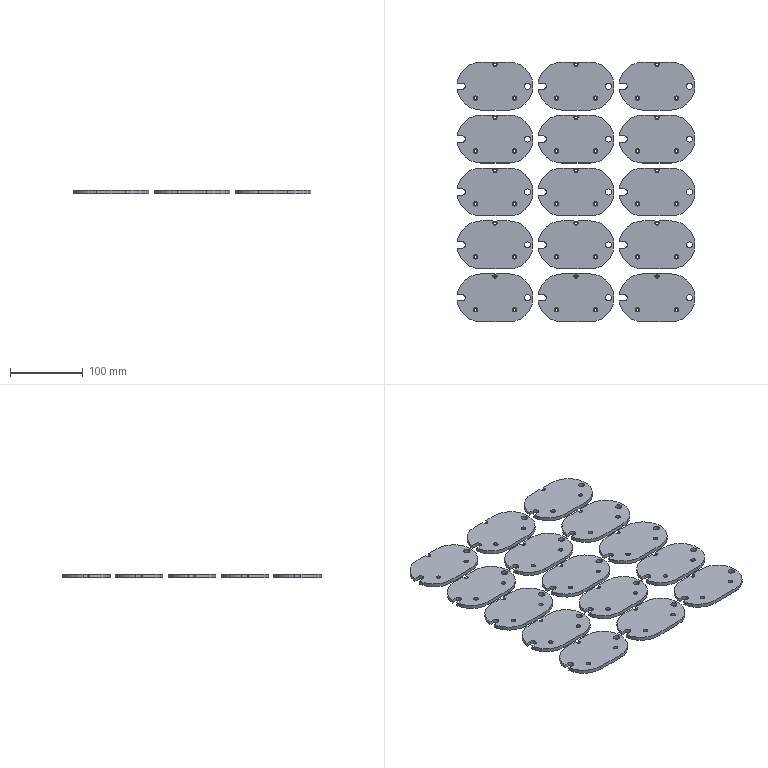NC program | NX | posted with a generic post | part box 328.125 x 358 x 5 mm
Lines 5444 to 6263 of 9242:
(HOLE_MILLING , TOOL : D4)
N10886 T04 M6
N10888 G54
N10890 G17 G0 G90 X-129.5 Y138.409 S7500 M3
N10892 G43 Z30. H4
N10894 Z0.5
N10896 G94 G3 X-129. Y138.909 R0.5 F1350.
N10898 X-129.5 Y139.409 R0.5
N10900 X-129.5 Y139.409 Z0.15 I0. J-1.
N10902 X-129.5 Y139.409 Z-0.2 I0. J-1.
N10904 X-129.5 Y139.409 Z-0.55 I0. J-1.
N10906 X-129.5 Y139.409 Z-0.9 I0. J-1.
N10908 X-129.5 Y139.409 Z-1.25 I0. J-1.
N10910 X-129.5 Y139.409 Z-1.6 I0. J-1.
N10912 X-129.5 Y139.409 Z-1.95 I0. J-1.
N10914 X-129.5 Y139.409 Z-2.3 I0. J-1.
N10916 X-129.5 Y139.409 Z-2.65 I0. J-1.
N10918 X-129.5 Y139.409 Z-3. I0. J-1.
N10920 X-130.5 Y138.409 R1.
N10922 X-129.5 Y139.409 R-1.
N10924 X-130. Y138.909 R0.5
N10926 X-129.5 Y138.409 R0.5
N10928 G0 Z30.
N10930 Y84.716
N10932 Z0.5
N10934 G3 X-129. Y85.216 R0.5
N10936 X-129.5 Y85.716 R0.5
N10938 X-129.5 Y85.716 Z0.15 I0. J-1.
N10940 X-129.5 Y85.716 Z-0.2 I0. J-1.
N10942 X-129.5 Y85.716 Z-0.55 I0. J-1.
N10944 X-129.5 Y85.716 Z-0.9 I0. J-1.
N10946 X-129.5 Y85.716 Z-1.25 I0. J-1.
N10948 X-129.5 Y85.716 Z-1.6 I0. J-1.
N10950 X-129.5 Y85.716 Z-1.95 I0. J-1.
N10952 X-129.5 Y85.716 Z-2.3 I0. J-1.
N10954 X-129.5 Y85.716 Z-2.65 I0. J-1.
N10956 X-129.5 Y85.716 Z-3. I0. J-1.
N10958 X-130.5 Y84.716 R1.
N10960 X-129.5 Y85.716 R-1.
N10962 X-130. Y85.216 R0.5
N10964 X-129.5 Y84.716 R0.5
N10966 G0 Z30.
N10968 Y26.709
N10970 Z0.5
N10972 G3 X-129. Y27.209 R0.5
N10974 X-129.5 Y27.709 R0.5
N10976 X-129.5 Y27.709 Z0.15 I0. J-1.
N10978 X-129.5 Y27.709 Z-0.2 I0. J-1.
N10980 X-129.5 Y27.709 Z-0.55 I0. J-1.
N10982 X-129.5 Y27.709 Z-0.9 I0. J-1.
N10984 X-129.5 Y27.709 Z-1.25 I0. J-1.
N10986 X-129.5 Y27.709 Z-1.6 I0. J-1.
N10988 X-129.5 Y27.709 Z-1.95 I0. J-1.
N10990 X-129.5 Y27.709 Z-2.3 I0. J-1.
N10992 X-129.5 Y27.709 Z-2.65 I0. J-1.
N10994 X-129.5 Y27.709 Z-3. I0. J-1.
N10996 X-130.5 Y26.709 R1.
N10998 X-129.5 Y27.709 R-1.
N11000 X-130. Y27.209 R0.5
N11002 X-129.5 Y26.709 R0.5
N11004 G0 Z30.
N11006 Y-26.984
N11008 Z0.5
N11010 G3 X-129. Y-26.484 R0.5
N11012 X-129.5 Y-25.984 R0.5
N11014 X-129.5 Y-25.984 Z0.15 I0. J-1.
N11016 X-129.5 Y-25.984 Z-0.2 I0. J-1.
N11018 X-129.5 Y-25.984 Z-0.55 I0. J-1.
N11020 X-129.5 Y-25.984 Z-0.9 I0. J-1.
N11022 X-129.5 Y-25.984 Z-1.25 I0. J-1.
N11024 X-129.5 Y-25.984 Z-1.6 I0. J-1.
N11026 X-129.5 Y-25.984 Z-1.95 I0. J-1.
N11028 X-129.5 Y-25.984 Z-2.3 I0. J-1.
N11030 X-129.5 Y-25.984 Z-2.65 I0. J-1.
N11032 X-129.5 Y-25.984 Z-3. I0. J-1.
N11034 X-130.5 Y-26.984 R1.
N11036 X-129.5 Y-25.984 R-1.
N11038 X-130. Y-26.484 R0.5
N11040 X-129.5 Y-26.984 R0.5
N11042 G0 Z30.
N11044 Y-84.991
N11046 Z0.5
N11048 G3 X-129. Y-84.491 R0.5
N11050 X-129.5 Y-83.991 R0.5
N11052 X-129.5 Y-83.991 Z0.15 I0. J-1.
N11054 X-129.5 Y-83.991 Z-0.2 I0. J-1.
N11056 X-129.5 Y-83.991 Z-0.55 I0. J-1.
N11058 X-129.5 Y-83.991 Z-0.9 I0. J-1.
N11060 X-129.5 Y-83.991 Z-1.25 I0. J-1.
N11062 X-129.5 Y-83.991 Z-1.6 I0. J-1.
N11064 X-129.5 Y-83.991 Z-1.95 I0. J-1.
N11066 X-129.5 Y-83.991 Z-2.3 I0. J-1.
N11068 X-129.5 Y-83.991 Z-2.65 I0. J-1.
N11070 X-129.5 Y-83.991 Z-3. I0. J-1.
N11072 X-130.5 Y-84.991 R1.
N11074 X-129.5 Y-83.991 R-1.
N11076 X-130. Y-84.491 R0.5
N11078 X-129.5 Y-84.991 R0.5
N11080 G0 Z30.
N11082 Y-138.684
N11084 Z0.5
N11086 G3 X-129. Y-138.184 R0.5
N11088 X-129.5 Y-137.684 R0.5
N11090 X-129.5 Y-137.684 Z0.15 I0. J-1.
N11092 X-129.5 Y-137.684 Z-0.2 I0. J-1.
N11094 X-129.5 Y-137.684 Z-0.55 I0. J-1.
N11096 X-129.5 Y-137.684 Z-0.9 I0. J-1.
N11098 X-129.5 Y-137.684 Z-1.25 I0. J-1.
N11100 X-129.5 Y-137.684 Z-1.6 I0. J-1.
N11102 X-129.5 Y-137.684 Z-1.95 I0. J-1.
N11104 X-129.5 Y-137.684 Z-2.3 I0. J-1.
N11106 X-129.5 Y-137.684 Z-2.65 I0. J-1.
N11108 X-129.5 Y-137.684 Z-3. I0. J-1.
N11110 X-130.5 Y-138.684 R1.
N11112 X-129.5 Y-137.684 R-1.
N11114 X-130. Y-138.184 R0.5
N11116 X-129.5 Y-138.684 R0.5
N11118 G0 Z30.
N11120 X-56.5
N11122 Z0.5
N11124 G3 X-56. Y-138.184 R0.5
N11126 X-56.5 Y-137.684 R0.5
N11128 X-56.5 Y-137.684 Z0.15 I0. J-1.
N11130 X-56.5 Y-137.684 Z-0.2 I0. J-1.
N11132 X-56.5 Y-137.684 Z-0.55 I0. J-1.
N11134 X-56.5 Y-137.684 Z-0.9 I0. J-1.
N11136 X-56.5 Y-137.684 Z-1.25 I0. J-1.
N11138 X-56.5 Y-137.684 Z-1.6 I0. J-1.
N11140 X-56.5 Y-137.684 Z-1.95 I0. J-1.
N11142 X-56.5 Y-137.684 Z-2.3 I0. J-1.
N11144 X-56.5 Y-137.684 Z-2.65 I0. J-1.
N11146 X-56.5 Y-137.684 Z-3. I0. J-1.
N11148 X-57.5 Y-138.684 R1.
N11150 X-56.5 Y-137.684 R-1.
N11152 X-57. Y-138.184 R0.5
N11154 X-56.5 Y-138.684 R0.5
N11156 G0 Z30.
N11158 Y-84.991
N11160 Z0.5
N11162 G3 X-56. Y-84.491 R0.5
N11164 X-56.5 Y-83.991 R0.5
N11166 X-56.5 Y-83.991 Z0.15 I0. J-1.
N11168 X-56.5 Y-83.991 Z-0.2 I0. J-1.
N11170 X-56.5 Y-83.991 Z-0.55 I0. J-1.
N11172 X-56.5 Y-83.991 Z-0.9 I0. J-1.
N11174 X-56.5 Y-83.991 Z-1.25 I0. J-1.
N11176 X-56.5 Y-83.991 Z-1.6 I0. J-1.
N11178 X-56.5 Y-83.991 Z-1.95 I0. J-1.
N11180 X-56.5 Y-83.991 Z-2.3 I0. J-1.
N11182 X-56.5 Y-83.991 Z-2.65 I0. J-1.
N11184 X-56.5 Y-83.991 Z-3. I0. J-1.
N11186 X-57.5 Y-84.991 R1.
N11188 X-56.5 Y-83.991 R-1.
N11190 X-57. Y-84.491 R0.5
N11192 X-56.5 Y-84.991 R0.5
N11194 G0 Z30.
N11196 Y-26.984
N11198 Z0.5
N11200 G3 X-56. Y-26.484 R0.5
N11202 X-56.5 Y-25.984 R0.5
N11204 X-56.5 Y-25.984 Z0.15 I0. J-1.
N11206 X-56.5 Y-25.984 Z-0.2 I0. J-1.
N11208 X-56.5 Y-25.984 Z-0.55 I0. J-1.
N11210 X-56.5 Y-25.984 Z-0.9 I0. J-1.
N11212 X-56.5 Y-25.984 Z-1.25 I0. J-1.
N11214 X-56.5 Y-25.984 Z-1.6 I0. J-1.
N11216 X-56.5 Y-25.984 Z-1.95 I0. J-1.
N11218 X-56.5 Y-25.984 Z-2.3 I0. J-1.
N11220 X-56.5 Y-25.984 Z-2.65 I0. J-1.
N11222 X-56.5 Y-25.984 Z-3. I0. J-1.
N11224 X-57.5 Y-26.984 R1.
N11226 X-56.5 Y-25.984 R-1.
N11228 X-57. Y-26.484 R0.5
N11230 X-56.5 Y-26.984 R0.5
N11232 G0 Z30.
N11234 Y26.709
N11236 Z0.5
N11238 G3 X-56. Y27.209 R0.5
N11240 X-56.5 Y27.709 R0.5
N11242 X-56.5 Y27.709 Z0.15 I0. J-1.
N11244 X-56.5 Y27.709 Z-0.2 I0. J-1.
N11246 X-56.5 Y27.709 Z-0.55 I0. J-1.
N11248 X-56.5 Y27.709 Z-0.9 I0. J-1.
N11250 X-56.5 Y27.709 Z-1.25 I0. J-1.
N11252 X-56.5 Y27.709 Z-1.6 I0. J-1.
N11254 X-56.5 Y27.709 Z-1.95 I0. J-1.
N11256 X-56.5 Y27.709 Z-2.3 I0. J-1.
N11258 X-56.5 Y27.709 Z-2.65 I0. J-1.
N11260 X-56.5 Y27.709 Z-3. I0. J-1.
N11262 X-57.5 Y26.709 R1.
N11264 X-56.5 Y27.709 R-1.
N11266 X-57. Y27.209 R0.5
N11268 X-56.5 Y26.709 R0.5
N11270 G0 Z30.
N11272 Y84.716
N11274 Z0.5
N11276 G3 X-56. Y85.216 R0.5
N11278 X-56.5 Y85.716 R0.5
N11280 X-56.5 Y85.716 Z0.15 I0. J-1.
N11282 X-56.5 Y85.716 Z-0.2 I0. J-1.
N11284 X-56.5 Y85.716 Z-0.55 I0. J-1.
N11286 X-56.5 Y85.716 Z-0.9 I0. J-1.
N11288 X-56.5 Y85.716 Z-1.25 I0. J-1.
N11290 X-56.5 Y85.716 Z-1.6 I0. J-1.
N11292 X-56.5 Y85.716 Z-1.95 I0. J-1.
N11294 X-56.5 Y85.716 Z-2.3 I0. J-1.
N11296 X-56.5 Y85.716 Z-2.65 I0. J-1.
N11298 X-56.5 Y85.716 Z-3. I0. J-1.
N11300 X-57.5 Y84.716 R1.
N11302 X-56.5 Y85.716 R-1.
N11304 X-57. Y85.216 R0.5
N11306 X-56.5 Y84.716 R0.5
N11308 G0 Z30.
N11310 Y138.409
N11312 Z0.5
N11314 G3 X-56. Y138.909 R0.5
N11316 X-56.5 Y139.409 R0.5
N11318 X-56.5 Y139.409 Z0.15 I0. J-1.
N11320 X-56.5 Y139.409 Z-0.2 I0. J-1.
N11322 X-56.5 Y139.409 Z-0.55 I0. J-1.
N11324 X-56.5 Y139.409 Z-0.9 I0. J-1.
N11326 X-56.5 Y139.409 Z-1.25 I0. J-1.
N11328 X-56.5 Y139.409 Z-1.6 I0. J-1.
N11330 X-56.5 Y139.409 Z-1.95 I0. J-1.
N11332 X-56.5 Y139.409 Z-2.3 I0. J-1.
N11334 X-56.5 Y139.409 Z-2.65 I0. J-1.
N11336 X-56.5 Y139.409 Z-3. I0. J-1.
N11338 X-57.5 Y138.409 R1.
N11340 X-56.5 Y139.409 R-1.
N11342 X-57. Y138.909 R0.5
N11344 X-56.5 Y138.409 R0.5
N11346 G0 Z30.
N11348 X16.5
N11350 Z0.5
N11352 G3 X17. Y138.909 R0.5
N11354 X16.5 Y139.409 R0.5
N11356 X16.5 Y139.409 Z0.15 I0. J-1.
N11358 X16.5 Y139.409 Z-0.2 I0. J-1.
N11360 X16.5 Y139.409 Z-0.55 I0. J-1.
N11362 X16.5 Y139.409 Z-0.9 I0. J-1.
N11364 X16.5 Y139.409 Z-1.25 I0. J-1.
N11366 X16.5 Y139.409 Z-1.6 I0. J-1.
N11368 X16.5 Y139.409 Z-1.95 I0. J-1.
N11370 X16.5 Y139.409 Z-2.3 I0. J-1.
N11372 X16.5 Y139.409 Z-2.65 I0. J-1.
N11374 X16.5 Y139.409 Z-3. I0. J-1.
N11376 X15.5 Y138.409 R1.
N11378 X16.5 Y139.409 R-1.
N11380 X16. Y138.909 R0.5
N11382 X16.5 Y138.409 R0.5
N11384 G0 Z30.
N11386 Y84.716
N11388 Z0.5
N11390 G3 X17. Y85.216 R0.5
N11392 X16.5 Y85.716 R0.5
N11394 X16.5 Y85.716 Z0.15 I0. J-1.
N11396 X16.5 Y85.716 Z-0.2 I0. J-1.
N11398 X16.5 Y85.716 Z-0.55 I0. J-1.
N11400 X16.5 Y85.716 Z-0.9 I0. J-1.
N11402 X16.5 Y85.716 Z-1.25 I0. J-1.
N11404 X16.5 Y85.716 Z-1.6 I0. J-1.
N11406 X16.5 Y85.716 Z-1.95 I0. J-1.
N11408 X16.5 Y85.716 Z-2.3 I0. J-1.
N11410 X16.5 Y85.716 Z-2.65 I0. J-1.
N11412 X16.5 Y85.716 Z-3. I0. J-1.
N11414 X15.5 Y84.716 R1.
N11416 X16.5 Y85.716 R-1.
N11418 X16. Y85.216 R0.5
N11420 X16.5 Y84.716 R0.5
N11422 G0 Z30.
N11424 Y26.709
N11426 Z0.5
N11428 G3 X17. Y27.209 R0.5
N11430 X16.5 Y27.709 R0.5
N11432 X16.5 Y27.709 Z0.15 I0. J-1.
N11434 X16.5 Y27.709 Z-0.2 I0. J-1.
N11436 X16.5 Y27.709 Z-0.55 I0. J-1.
N11438 X16.5 Y27.709 Z-0.9 I0. J-1.
N11440 X16.5 Y27.709 Z-1.25 I0. J-1.
N11442 X16.5 Y27.709 Z-1.6 I0. J-1.
N11444 X16.5 Y27.709 Z-1.95 I0. J-1.
N11446 X16.5 Y27.709 Z-2.3 I0. J-1.
N11448 X16.5 Y27.709 Z-2.65 I0. J-1.
N11450 X16.5 Y27.709 Z-3. I0. J-1.
N11452 X15.5 Y26.709 R1.
N11454 X16.5 Y27.709 R-1.
N11456 X16. Y27.209 R0.5
N11458 X16.5 Y26.709 R0.5
N11460 G0 Z30.
N11462 Y-26.984
N11464 Z0.5
N11466 G3 X17. Y-26.484 R0.5
N11468 X16.5 Y-25.984 R0.5
N11470 X16.5 Y-25.984 Z0.15 I0. J-1.
N11472 X16.5 Y-25.984 Z-0.2 I0. J-1.
N11474 X16.5 Y-25.984 Z-0.55 I0. J-1.
N11476 X16.5 Y-25.984 Z-0.9 I0. J-1.
N11478 X16.5 Y-25.984 Z-1.25 I0. J-1.
N11480 X16.5 Y-25.984 Z-1.6 I0. J-1.
N11482 X16.5 Y-25.984 Z-1.95 I0. J-1.
N11484 X16.5 Y-25.984 Z-2.3 I0. J-1.
N11486 X16.5 Y-25.984 Z-2.65 I0. J-1.
N11488 X16.5 Y-25.984 Z-3. I0. J-1.
N11490 X15.5 Y-26.984 R1.
N11492 X16.5 Y-25.984 R-1.
N11494 X16. Y-26.484 R0.5
N11496 X16.5 Y-26.984 R0.5
N11498 G0 Z30.
N11500 Y-84.991
N11502 Z0.5
N11504 G3 X17. Y-84.491 R0.5
N11506 X16.5 Y-83.991 R0.5
N11508 X16.5 Y-83.991 Z0.15 I0. J-1.
N11510 X16.5 Y-83.991 Z-0.2 I0. J-1.
N11512 X16.5 Y-83.991 Z-0.55 I0. J-1.
N11514 X16.5 Y-83.991 Z-0.9 I0. J-1.
N11516 X16.5 Y-83.991 Z-1.25 I0. J-1.
N11518 X16.5 Y-83.991 Z-1.6 I0. J-1.
N11520 X16.5 Y-83.991 Z-1.95 I0. J-1.
N11522 X16.5 Y-83.991 Z-2.3 I0. J-1.
N11524 X16.5 Y-83.991 Z-2.65 I0. J-1.
N11526 X16.5 Y-83.991 Z-3. I0. J-1.
N11528 X15.5 Y-84.991 R1.
N11530 X16.5 Y-83.991 R-1.
N11532 X16. Y-84.491 R0.5
N11534 X16.5 Y-84.991 R0.5
N11536 G0 Z30.
N11538 Y-138.684
N11540 Z0.5
N11542 G3 X17. Y-138.184 R0.5
N11544 X16.5 Y-137.684 R0.5
N11546 X16.5 Y-137.684 Z0.15 I0. J-1.
N11548 X16.5 Y-137.684 Z-0.2 I0. J-1.
N11550 X16.5 Y-137.684 Z-0.55 I0. J-1.
N11552 X16.5 Y-137.684 Z-0.9 I0. J-1.
N11554 X16.5 Y-137.684 Z-1.25 I0. J-1.
N11556 X16.5 Y-137.684 Z-1.6 I0. J-1.
N11558 X16.5 Y-137.684 Z-1.95 I0. J-1.
N11560 X16.5 Y-137.684 Z-2.3 I0. J-1.
N11562 X16.5 Y-137.684 Z-2.65 I0. J-1.
N11564 X16.5 Y-137.684 Z-3. I0. J-1.
N11566 X15.5 Y-138.684 R1.
N11568 X16.5 Y-137.684 R-1.
N11570 X16. Y-138.184 R0.5
N11572 X16.5 Y-138.684 R0.5
N11574 G0 Z30.
N11576 X89.5
N11578 Z0.5
N11580 G3 X90. Y-138.184 R0.5
N11582 X89.5 Y-137.684 R0.5
N11584 X89.5 Y-137.684 Z0.15 I0. J-1.
N11586 X89.5 Y-137.684 Z-0.2 I0. J-1.
N11588 X89.5 Y-137.684 Z-0.55 I0. J-1.
N11590 X89.5 Y-137.684 Z-0.9 I0. J-1.
N11592 X89.5 Y-137.684 Z-1.25 I0. J-1.
N11594 X89.5 Y-137.684 Z-1.6 I0. J-1.
N11596 X89.5 Y-137.684 Z-1.95 I0. J-1.
N11598 X89.5 Y-137.684 Z-2.3 I0. J-1.
N11600 X89.5 Y-137.684 Z-2.65 I0. J-1.
N11602 X89.5 Y-137.684 Z-3. I0. J-1.
N11604 X88.5 Y-138.684 R1.
N11606 X89.5 Y-137.684 R-1.
N11608 X89. Y-138.184 R0.5
N11610 X89.5 Y-138.684 R0.5
N11612 G0 Z30.
N11614 Y-84.991
N11616 Z0.5
N11618 G3 X90. Y-84.491 R0.5
N11620 X89.5 Y-83.991 R0.5
N11622 X89.5 Y-83.991 Z0.15 I0. J-1.
N11624 X89.5 Y-83.991 Z-0.2 I0. J-1.
N11626 X89.5 Y-83.991 Z-0.55 I0. J-1.
N11628 X89.5 Y-83.991 Z-0.9 I0. J-1.
N11630 X89.5 Y-83.991 Z-1.25 I0. J-1.
N11632 X89.5 Y-83.991 Z-1.6 I0. J-1.
N11634 X89.5 Y-83.991 Z-1.95 I0. J-1.
N11636 X89.5 Y-83.991 Z-2.3 I0. J-1.
N11638 X89.5 Y-83.991 Z-2.65 I0. J-1.
N11640 X89.5 Y-83.991 Z-3. I0. J-1.
N11642 X88.5 Y-84.991 R1.
N11644 X89.5 Y-83.991 R-1.
N11646 X89. Y-84.491 R0.5
N11648 X89.5 Y-84.991 R0.5
N11650 G0 Z30.
N11652 Y-26.984
N11654 Z0.5
N11656 G3 X90. Y-26.484 R0.5
N11658 X89.5 Y-25.984 R0.5
N11660 X89.5 Y-25.984 Z0.15 I0. J-1.
N11662 X89.5 Y-25.984 Z-0.2 I0. J-1.
N11664 X89.5 Y-25.984 Z-0.55 I0. J-1.
N11666 X89.5 Y-25.984 Z-0.9 I0. J-1.
N11668 X89.5 Y-25.984 Z-1.25 I0. J-1.
N11670 X89.5 Y-25.984 Z-1.6 I0. J-1.
N11672 X89.5 Y-25.984 Z-1.95 I0. J-1.
N11674 X89.5 Y-25.984 Z-2.3 I0. J-1.
N11676 X89.5 Y-25.984 Z-2.65 I0. J-1.
N11678 X89.5 Y-25.984 Z-3. I0. J-1.
N11680 X88.5 Y-26.984 R1.
N11682 X89.5 Y-25.984 R-1.
N11684 X89. Y-26.484 R0.5
N11686 X89.5 Y-26.984 R0.5
N11688 G0 Z30.
N11690 Y26.709
N11692 Z0.5
N11694 G3 X90. Y27.209 R0.5
N11696 X89.5 Y27.709 R0.5
N11698 X89.5 Y27.709 Z0.15 I0. J-1.
N11700 X89.5 Y27.709 Z-0.2 I0. J-1.
N11702 X89.5 Y27.709 Z-0.55 I0. J-1.
N11704 X89.5 Y27.709 Z-0.9 I0. J-1.
N11706 X89.5 Y27.709 Z-1.25 I0. J-1.
N11708 X89.5 Y27.709 Z-1.6 I0. J-1.
N11710 X89.5 Y27.709 Z-1.95 I0. J-1.
N11712 X89.5 Y27.709 Z-2.3 I0. J-1.
N11714 X89.5 Y27.709 Z-2.65 I0. J-1.
N11716 X89.5 Y27.709 Z-3. I0. J-1.
N11718 X88.5 Y26.709 R1.
N11720 X89.5 Y27.709 R-1.
N11722 X89. Y27.209 R0.5
N11724 X89.5 Y26.709 R0.5
N11726 G0 Z30.
N11728 Y84.716
N11730 Z0.5
N11732 G3 X90. Y85.216 R0.5
N11734 X89.5 Y85.716 R0.5
N11736 X89.5 Y85.716 Z0.15 I0. J-1.
N11738 X89.5 Y85.716 Z-0.2 I0. J-1.
N11740 X89.5 Y85.716 Z-0.55 I0. J-1.
N11742 X89.5 Y85.716 Z-0.9 I0. J-1.
N11744 X89.5 Y85.716 Z-1.25 I0. J-1.
N11746 X89.5 Y85.716 Z-1.6 I0. J-1.
N11748 X89.5 Y85.716 Z-1.95 I0. J-1.
N11750 X89.5 Y85.716 Z-2.3 I0. J-1.
N11752 X89.5 Y85.716 Z-2.65 I0. J-1.
N11754 X89.5 Y85.716 Z-3. I0. J-1.
N11756 X88.5 Y84.716 R1.
N11758 X89.5 Y85.716 R-1.
N11760 X89. Y85.216 R0.5
N11762 X89.5 Y84.716 R0.5
N11764 G0 Z30.
N11766 Y138.409
N11768 Z0.5
N11770 G3 X90. Y138.909 R0.5
N11772 X89.5 Y139.409 R0.5
N11774 X89.5 Y139.409 Z0.15 I0. J-1.
N11776 X89.5 Y139.409 Z-0.2 I0. J-1.
N11778 X89.5 Y139.409 Z-0.55 I0. J-1.
N11780 X89.5 Y139.409 Z-0.9 I0. J-1.
N11782 X89.5 Y139.409 Z-1.25 I0. J-1.
N11784 X89.5 Y139.409 Z-1.6 I0. J-1.
N11786 X89.5 Y139.409 Z-1.95 I0. J-1.
N11788 X89.5 Y139.409 Z-2.3 I0. J-1.
N11790 X89.5 Y139.409 Z-2.65 I0. J-1.
N11792 X89.5 Y139.409 Z-3. I0. J-1.
N11794 X88.5 Y138.409 R1.
N11796 X89.5 Y139.409 R-1.
N11798 X89. Y138.909 R0.5
N11800 X89.5 Y138.409 R0.5
N11802 G0 Z30.
N11804 X162.5
N11806 Z0.5
N11808 G3 X163. Y138.909 R0.5
N11810 X162.5 Y139.409 R0.5
N11812 X162.5 Y139.409 Z0.15 I0. J-1.
N11814 X162.5 Y139.409 Z-0.2 I0. J-1.
N11816 X162.5 Y139.409 Z-0.55 I0. J-1.
N11818 X162.5 Y139.409 Z-0.9 I0. J-1.
N11820 X162.5 Y139.409 Z-1.25 I0. J-1.
N11822 X162.5 Y139.409 Z-1.6 I0. J-1.
N11824 X162.5 Y139.409 Z-1.95 I0. J-1.
N11826 X162.5 Y139.409 Z-2.3 I0. J-1.
N11828 X162.5 Y139.409 Z-2.65 I0. J-1.
N11830 X162.5 Y139.409 Z-3. I0. J-1.
N11832 X161.5 Y138.409 R1.
N11834 X162.5 Y139.409 R-1.
N11836 X162. Y138.909 R0.5
N11838 X162.5 Y138.409 R0.5
N11840 G0 Z30.
N11842 Y84.716
N11844 Z0.5
N11846 G3 X163. Y85.216 R0.5
N11848 X162.5 Y85.716 R0.5
N11850 X162.5 Y85.716 Z0.15 I0. J-1.
N11852 X162.5 Y85.716 Z-0.2 I0. J-1.
N11854 X162.5 Y85.716 Z-0.55 I0. J-1.
N11856 X162.5 Y85.716 Z-0.9 I0. J-1.
N11858 X162.5 Y85.716 Z-1.25 I0. J-1.
N11860 X162.5 Y85.716 Z-1.6 I0. J-1.
N11862 X162.5 Y85.716 Z-1.95 I0. J-1.
N11864 X162.5 Y85.716 Z-2.3 I0. J-1.
N11866 X162.5 Y85.716 Z-2.65 I0. J-1.
N11868 X162.5 Y85.716 Z-3. I0. J-1.
N11870 X161.5 Y84.716 R1.
N11872 X162.5 Y85.716 R-1.
N11874 X162. Y85.216 R0.5
N11876 X162.5 Y84.716 R0.5
N11878 G0 Z30.
N11880 Y26.709
N11882 Z0.5
N11884 G3 X163. Y27.209 R0.5
N11886 X162.5 Y27.709 R0.5
N11888 X162.5 Y27.709 Z0.15 I0. J-1.
N11890 X162.5 Y27.709 Z-0.2 I0. J-1.
N11892 X162.5 Y27.709 Z-0.55 I0. J-1.
N11894 X162.5 Y27.709 Z-0.9 I0. J-1.
N11896 X162.5 Y27.709 Z-1.25 I0. J-1.
N11898 X162.5 Y27.709 Z-1.6 I0. J-1.
N11900 X162.5 Y27.709 Z-1.95 I0. J-1.
N11902 X162.5 Y27.709 Z-2.3 I0. J-1.
N11904 X162.5 Y27.709 Z-2.65 I0. J-1.
N11906 X162.5 Y27.709 Z-3. I0. J-1.
N11908 X161.5 Y26.709 R1.
N11910 X162.5 Y27.709 R-1.
N11912 X162. Y27.209 R0.5
N11914 X162.5 Y26.709 R0.5
N11916 G0 Z30.
N11918 Y-26.984
N11920 Z0.5
N11922 G3 X163. Y-26.484 R0.5
N11924 X162.5 Y-25.984 R0.5
N11926 X162.5 Y-25.984 Z0.15 I0. J-1.
N11928 X162.5 Y-25.984 Z-0.2 I0. J-1.
N11930 X162.5 Y-25.984 Z-0.55 I0. J-1.
N11932 X162.5 Y-25.984 Z-0.9 I0. J-1.
N11934 X162.5 Y-25.984 Z-1.25 I0. J-1.
N11936 X162.5 Y-25.984 Z-1.6 I0. J-1.
N11938 X162.5 Y-25.984 Z-1.95 I0. J-1.
N11940 X162.5 Y-25.984 Z-2.3 I0. J-1.
N11942 X162.5 Y-25.984 Z-2.65 I0. J-1.
N11944 X162.5 Y-25.984 Z-3. I0. J-1.
N11946 X161.5 Y-26.984 R1.
N11948 X162.5 Y-25.984 R-1.
N11950 X162. Y-26.484 R0.5
N11952 X162.5 Y-26.984 R0.5
N11954 G0 Z30.
N11956 Y-84.991
N11958 Z0.5
N11960 G3 X163. Y-84.491 R0.5
N11962 X162.5 Y-83.991 R0.5
N11964 X162.5 Y-83.991 Z0.15 I0. J-1.
N11966 X162.5 Y-83.991 Z-0.2 I0. J-1.
N11968 X162.5 Y-83.991 Z-0.55 I0. J-1.
N11970 X162.5 Y-83.991 Z-0.9 I0. J-1.
N11972 X162.5 Y-83.991 Z-1.25 I0. J-1.
N11974 X162.5 Y-83.991 Z-1.6 I0. J-1.
N11976 X162.5 Y-83.991 Z-1.95 I0. J-1.
N11978 X162.5 Y-83.991 Z-2.3 I0. J-1.
N11980 X162.5 Y-83.991 Z-2.65 I0. J-1.
N11982 X162.5 Y-83.991 Z-3. I0. J-1.
N11984 X161.5 Y-84.991 R1.
N11986 X162.5 Y-83.991 R-1.
N11988 X162. Y-84.491 R0.5
N11990 X162.5 Y-84.991 R0.5
N11992 G0 Z30.
N11994 Y-138.684
N11996 Z0.5
N11998 G3 X163. Y-138.184 R0.5
N12000 X162.5 Y-137.684 R0.5
N12002 X162.5 Y-137.684 Z0.15 I0. J-1.
N12004 X162.5 Y-137.684 Z-0.2 I0. J-1.
N12006 X162.5 Y-137.684 Z-0.55 I0. J-1.
N12008 X162.5 Y-137.684 Z-0.9 I0. J-1.
N12010 X162.5 Y-137.684 Z-1.25 I0. J-1.
N12012 X162.5 Y-137.684 Z-1.6 I0. J-1.
N12014 X162.5 Y-137.684 Z-1.95 I0. J-1.
N12016 X162.5 Y-137.684 Z-2.3 I0. J-1.
N12018 X162.5 Y-137.684 Z-2.65 I0. J-1.
N12020 X162.5 Y-137.684 Z-3. I0. J-1.
N12022 X161.5 Y-138.684 R1.
N12024 X162.5 Y-137.684 R-1.
N12026 X162. Y-138.184 R0.5
N12028 X162.5 Y-138.684 R0.5
N12030 G0 Z30.
(ZLEVEL_PROFILE_1 , TOOL : D4)
N12032 X110.338 Y-112.12
N12034 Z-0.333
N12036 G1 X110.707 Y-112.667 F1500.
N12038 G3 X111.067 Y-112.842 R0.4
N12040 G1 X111.122 Y-112.838
N12042 X112.957 Y-112.837
N12044 X116.
N12046 G3 X117. Y-111.837 R1.
N12048 X116. Y-110.837 R1.
N12050 G1 X113.
N12052 X112.537 Y-110.783
N12054 X112.494 Y-110.836
N12056 X111.122
N12058 X111.067 Y-110.832
N12060 G3 X110.707 Y-111.008 R0.4
N12062 G1 X110.338 Y-111.555
N12064 G0 X110.331 Y-112.122 Z-0.667
N12066 G1 X110.699 Y-112.667
N12068 G3 X111.059 Y-112.843 R0.4
N12070 G1 X111.122 Y-112.838
N12072 X112.957 Y-112.837
N12074 X116.
N12076 G3 X117. Y-111.837 R1.
N12078 X116. Y-110.837 R1.
N12080 G1 X113.
N12082 X112.537 Y-110.783
N12084 X112.494 Y-110.837
N12086 X111.122
N12088 X111.059 Y-110.832
N12090 G3 X110.699 Y-111.007 R0.4
N12092 G1 X110.331 Y-111.553
N12094 G0 X110.324 Y-112.124 Z-1.
N12096 G1 X110.691 Y-112.668
N12098 G3 X111.051 Y-112.843 R0.4
N12100 G1 X111.122 Y-112.838
N12102 X112.957 Y-112.837
N12104 X116.
N12106 G3 X117. Y-111.837 R1.
N12108 X116. Y-110.837 R1.
N12110 G1 X113.
N12112 X112.537 Y-110.783
N12114 X112.494 Y-110.837
N12116 X111.122
N12118 X111.051 Y-110.832
N12120 G3 X110.691 Y-111.007 R0.4
N12122 G1 X110.324 Y-111.551
N12124 G0 X110.317 Y-112.126 Z-1.333
N12126 G1 X110.683 Y-112.668
N12128 G3 X111.043 Y-112.843 R0.4
N12130 G1 X111.122 Y-112.837
N12132 X112.957
N12134 X116.
N12136 G3 X117. Y-111.837 R1.
N12138 X116. Y-110.837 R1.
N12140 G1 X113.
N12142 X112.537 Y-110.783
N12144 X112.494 Y-110.837
N12146 X111.122
N12148 X111.043 Y-110.832
N12150 G3 X110.683 Y-111.007 R0.4
N12152 G1 X110.317 Y-111.549
N12154 G0 X110.31 Y-112.128 Z-1.667
N12156 G1 X110.675 Y-112.668
N12158 G3 X111.035 Y-112.843 R0.4
N12160 G1 X111.122 Y-112.837
N12162 X113.037
N12164 X116.
N12166 G3 X117. Y-111.837 R1.
N12168 X116. Y-110.837 R1.
N12170 G1 X113. Y-110.838
N12172 X112.537 Y-110.783
N12174 X112.494 Y-110.838
N12176 X111.122
N12178 X111.035 Y-110.832
N12180 G3 X110.675 Y-111.007 R0.4
N12182 G1 X110.31 Y-111.547
N12184 G0 X110.304 Y-112.13 Z-2.
N12186 G1 X110.667 Y-112.668
N12188 G3 X111.027 Y-112.844 R0.4
N12190 G1 X111.122 Y-112.837
N12192 X113.037
N12194 X116.
N12196 G3 X117. Y-111.837 R1.
N12198 X116. Y-110.837 R1.
N12200 G1 X113. Y-110.838
N12202 X112.537 Y-110.783
N12204 X112.494 Y-110.838
N12206 X111.122
N12208 X111.027 Y-110.831
N12210 G3 X110.667 Y-111.006 R0.4
N12212 G1 X110.304 Y-111.545
N12214 G0 X110.297 Y-112.132 Z-2.333
N12216 G1 X110.659 Y-112.669
N12218 G3 X111.019 Y-112.844 R0.4
N12220 G1 X111.122 Y-112.836
N12222 X113.037 Y-112.837
N12224 X116.
N12226 G3 X117. Y-111.837 R1.
N12228 X116. Y-110.837 R1.
N12230 G1 X113. Y-110.838
N12232 X112.537 Y-110.783
N12234 X112.494 Y-110.838
N12236 X111.122
N12238 X111.019 Y-110.831
N12240 G3 X110.659 Y-111.006 R0.4
N12242 G1 X110.297 Y-111.543
N12244 G0 X110.29 Y-112.134 Z-2.667
N12246 G1 X110.651 Y-112.669
N12248 G3 X111.011 Y-112.844 R0.4
N12250 G1 X111.122 Y-112.836
N12252 X113.037 Y-112.837
N12254 X116.
N12256 G3 X117. Y-111.837 R1.
N12258 X116. Y-110.837 R1.
N12260 G1 X113. Y-110.839
N12262 X112.537 Y-110.783
N12264 X112.494 Y-110.839
N12266 X111.122
N12268 X111.011 Y-110.831
N12270 G3 X110.651 Y-111.006 R0.4
N12272 G1 X110.29 Y-111.541
N12274 G0 X110.283 Y-112.136 Z-3.
N12276 G1 X110.643 Y-112.669
N12278 G3 X111.003 Y-112.844 R0.4
N12280 G1 X111.122 Y-112.836
N12282 X112.957 Y-112.838
N12284 X113.037 Y-112.837
N12286 X116.
N12288 G3 X117. Y-111.837 R1.
N12290 X116. Y-110.837 R1.
N12292 G1 X113. Y-110.839
N12294 X112.537 Y-110.783
N12296 X112.494 Y-110.839
N12298 X111.122
N12300 X111.003 Y-110.831
N12302 G3 X110.643 Y-111.006 R0.4
N12304 G1 X110.283 Y-111.539
N12306 G0 Z30.
N12308 X37.338 Y-112.12
N12310 Z-0.333
N12312 G1 X37.707 Y-112.667
N12314 G3 X38.067 Y-112.842 R0.4
N12316 G1 X38.122 Y-112.838
N12318 X39.948 Y-112.837
N12320 X43.
N12322 G3 X44. Y-111.837 R1.
N12324 X43. Y-110.837 R1.
N12326 G1 X40.
N12328 X39.537 Y-110.783
N12330 X39.494 Y-110.836
N12332 X38.122
N12334 X38.067 Y-110.832
N12336 G3 X37.707 Y-111.008 R0.4
N12338 G1 X37.338 Y-111.555
N12340 G0 X37.331 Y-112.122 Z-0.667
N12342 G1 X37.699 Y-112.667
N12344 G3 X38.059 Y-112.843 R0.4
N12346 G1 X38.122 Y-112.838
N12348 X39.948 Y-112.837
N12350 X43.
N12352 G3 X44. Y-111.837 R1.
N12354 X43. Y-110.837 R1.
N12356 G1 X40.
N12358 X39.537 Y-110.783
N12360 X39.494 Y-110.837
N12362 X38.122
N12364 X38.059 Y-110.832
N12366 G3 X37.699 Y-111.007 R0.4
N12368 G1 X37.331 Y-111.553
N12370 G0 X37.324 Y-112.124 Z-1.
N12372 G1 X37.691 Y-112.668
N12374 G3 X38.051 Y-112.843 R0.4
N12376 G1 X38.122 Y-112.838
N12378 X39.948 Y-112.837
N12380 X43.
N12382 G3 X44. Y-111.837 R1.
N12384 X43. Y-110.837 R1.
N12386 G1 X40.
N12388 X39.537 Y-110.783
N12390 X39.494 Y-110.837
N12392 X38.122
N12394 X38.051 Y-110.832
N12396 G3 X37.691 Y-111.007 R0.4
N12398 G1 X37.324 Y-111.551
N12400 G0 X37.317 Y-112.126 Z-1.333
N12402 G1 X37.683 Y-112.668
N12404 G3 X38.043 Y-112.843 R0.4
N12406 G1 X38.122 Y-112.837
N12408 X39.948
N12410 X43.
N12412 G3 X44. Y-111.837 R1.
N12414 X43. Y-110.837 R1.
N12416 G1 X40.
N12418 X39.537 Y-110.783
N12420 X39.494 Y-110.837
N12422 X38.122
N12424 X38.043 Y-110.832
N12426 G3 X37.683 Y-111.007 R0.4
N12428 G1 X37.317 Y-111.549
N12430 G0 X37.31 Y-112.128 Z-1.667
N12432 G1 X37.675 Y-112.668
N12434 G3 X38.035 Y-112.843 R0.4
N12436 G1 X38.122 Y-112.837
N12438 X40.037
N12440 X43.
N12442 G3 X44. Y-111.837 R1.
N12444 X43. Y-110.837 R1.
N12446 G1 X40. Y-110.838
N12448 X39.537 Y-110.783
N12450 X39.494 Y-110.838
N12452 X38.122
N12454 X38.035 Y-110.832
N12456 G3 X37.675 Y-111.007 R0.4
N12458 G1 X37.31 Y-111.547
N12460 G0 X37.304 Y-112.13 Z-2.
N12462 G1 X37.667 Y-112.668
N12464 G3 X38.027 Y-112.844 R0.4
N12466 G1 X38.122 Y-112.837
N12468 X40.037
N12470 X43.
N12472 G3 X44. Y-111.837 R1.
N12474 X43. Y-110.837 R1.
N12476 G1 X40. Y-110.838
N12478 X39.537 Y-110.783
N12480 X39.494 Y-110.838
N12482 X38.122
N12484 X38.027 Y-110.831
N12486 G3 X37.667 Y-111.006 R0.4
N12488 G1 X37.304 Y-111.545
N12490 G0 X37.297 Y-112.132 Z-2.333
N12492 G1 X37.659 Y-112.669
N12494 G3 X38.019 Y-112.844 R0.4
N12496 G1 X38.122 Y-112.836
N12498 X40.037 Y-112.837
N12500 X43.
N12502 G3 X44. Y-111.837 R1.
N12504 X43. Y-110.837 R1.
N12506 G1 X40. Y-110.838
N12508 X39.537 Y-110.783
N12510 X39.494 Y-110.838
N12512 X38.122